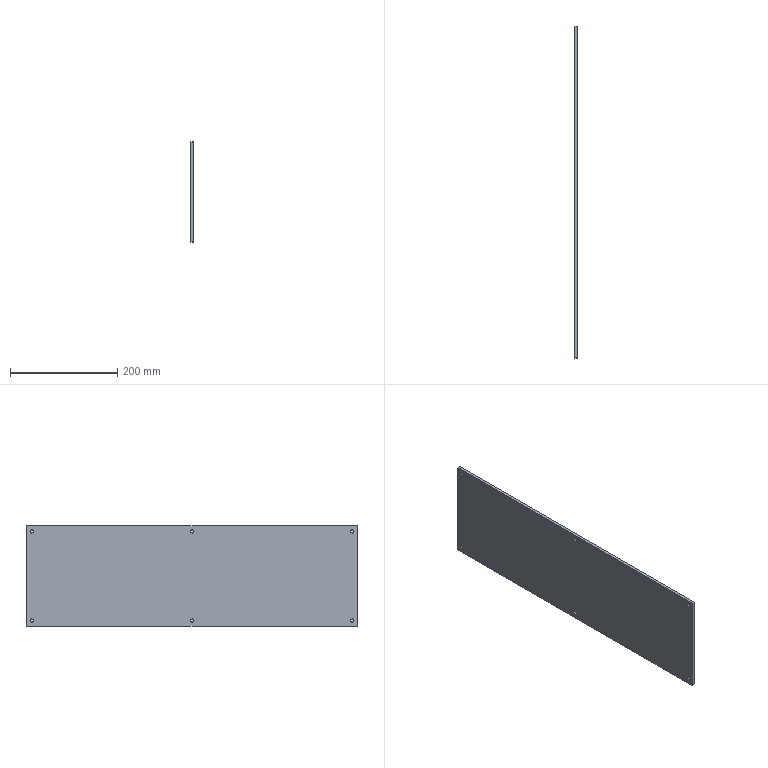Part | SolidWorks | features Chamfer 1, Extrusion 1, ICE 1 | 1 solid | 22 faces | box 5 x 618 x 188 mm | volume 580062 mm3 | cylinder 12 | plane 10 | commonest cylinder face diameters 6 x12
STEP:
#1=CARTESIAN_POINT('',(5.,0.,-86.));
#2=VERTEX_POINT('',#1);
#3=CARTESIAN_POINT('',(5.,0.,-80.));
#4=VERTEX_POINT('',#3);
#5=CARTESIAN_POINT('',(5.,0.,-83.));
#6=DIRECTION('',(-1.,0.,0.));
#7=DIRECTION('',(0.,0.,1.));
#8=AXIS2_PLACEMENT_3D('',#5,#6,#7);
#9=CIRCLE('',#8,3.);
#10=EDGE_CURVE('',#2,#4,#9,.T.);
#11=ORIENTED_EDGE('',*,*,#10,.F.);
#12=CARTESIAN_POINT('',(0.,0.,-86.));
#13=VERTEX_POINT('',#12);
#14=CARTESIAN_POINT('',(5.,0.,-86.));
#15=DIRECTION('',(-1.,0.,0.));
#16=VECTOR('',#15,1000.);
#17=LINE('',#14,#16);
#18=EDGE_CURVE('',#2,#13,#17,.T.);
#19=ORIENTED_EDGE('',*,*,#18,.T.);
#20=CARTESIAN_POINT('',(0.,0.,-80.));
#21=VERTEX_POINT('',#20);
#22=CARTESIAN_POINT('',(0.,0.,-83.));
#23=DIRECTION('',(-1.,0.,0.));
#24=DIRECTION('',(0.,0.,1.));
#25=AXIS2_PLACEMENT_3D('',#22,#23,#24);
#26=CIRCLE('',#25,3.);
#27=EDGE_CURVE('',#13,#21,#26,.T.);
#28=ORIENTED_EDGE('',*,*,#27,.T.);
#29=CARTESIAN_POINT('',(5.,0.,-80.));
#30=DIRECTION('',(-1.,0.,0.));
#31=VECTOR('',#30,1000.);
#32=LINE('',#29,#31);
#33=EDGE_CURVE('',#4,#21,#32,.T.);
#34=ORIENTED_EDGE('',*,*,#33,.F.);
#35=EDGE_LOOP('',(#11,#19,#28,#34));
#36=FACE_OUTER_BOUND('',#35,.T.);
#37=CARTESIAN_POINT('',(5.,0.,-83.));
#38=DIRECTION('',(-1.,0.,0.));
#39=DIRECTION('',(0.,0.,1.));
#40=AXIS2_PLACEMENT_3D('',#37,#38,#39);
#41=CYLINDRICAL_SURFACE('',#40,3.);
#42=ADVANCED_FACE('',(#36),#41,.F.);
#43=CARTESIAN_POINT('',(5.,0.,80.));
#44=VERTEX_POINT('',#43);
#45=CARTESIAN_POINT('',(5.,0.,86.));
#46=VERTEX_POINT('',#45);
#47=CARTESIAN_POINT('',(5.,0.,83.));
#48=DIRECTION('',(-1.,0.,0.));
#49=DIRECTION('',(0.,0.,1.));
#50=AXIS2_PLACEMENT_3D('',#47,#48,#49);
#51=CIRCLE('',#50,3.);
#52=EDGE_CURVE('',#44,#46,#51,.T.);
#53=ORIENTED_EDGE('',*,*,#52,.F.);
#54=CARTESIAN_POINT('',(0.,0.,80.));
#55=VERTEX_POINT('',#54);
#56=CARTESIAN_POINT('',(5.,0.,80.));
#57=DIRECTION('',(-1.,0.,0.));
#58=VECTOR('',#57,1000.);
#59=LINE('',#56,#58);
#60=EDGE_CURVE('',#44,#55,#59,.T.);
#61=ORIENTED_EDGE('',*,*,#60,.T.);
#62=CARTESIAN_POINT('',(0.,0.,86.));
#63=VERTEX_POINT('',#62);
#64=CARTESIAN_POINT('',(0.,0.,83.));
#65=DIRECTION('',(-1.,0.,0.));
#66=DIRECTION('',(0.,0.,1.));
#67=AXIS2_PLACEMENT_3D('',#64,#65,#66);
#68=CIRCLE('',#67,3.);
#69=EDGE_CURVE('',#55,#63,#68,.T.);
#70=ORIENTED_EDGE('',*,*,#69,.T.);
#71=CARTESIAN_POINT('',(5.,0.,86.));
#72=DIRECTION('',(-1.,0.,0.));
#73=VECTOR('',#72,1000.);
#74=LINE('',#71,#73);
#75=EDGE_CURVE('',#46,#63,#74,.T.);
#76=ORIENTED_EDGE('',*,*,#75,.F.);
#77=EDGE_LOOP('',(#53,#61,#70,#76));
#78=FACE_OUTER_BOUND('',#77,.T.);
#79=CARTESIAN_POINT('',(5.,0.,83.));
#80=DIRECTION('',(-1.,0.,0.));
#81=DIRECTION('',(0.,0.,1.));
#82=AXIS2_PLACEMENT_3D('',#79,#80,#81);
#83=CYLINDRICAL_SURFACE('',#82,3.);
#84=ADVANCED_FACE('',(#78),#83,.F.);
#85=CARTESIAN_POINT('',(5.,298.,80.));
#86=VERTEX_POINT('',#85);
#87=CARTESIAN_POINT('',(5.,298.,86.));
#88=VERTEX_POINT('',#87);
#89=CARTESIAN_POINT('',(5.,298.,83.));
#90=DIRECTION('',(-1.,0.,0.));
#91=DIRECTION('',(0.,0.,-1.));
#92=AXIS2_PLACEMENT_3D('',#89,#90,#91);
#93=CIRCLE('',#92,3.);
#94=EDGE_CURVE('',#86,#88,#93,.T.);
#95=ORIENTED_EDGE('',*,*,#94,.F.);
#96=CARTESIAN_POINT('',(0.,298.,80.));
#97=VERTEX_POINT('',#96);
#98=CARTESIAN_POINT('',(5.,298.,80.));
#99=DIRECTION('',(-1.,0.,0.));
#100=VECTOR('',#99,1000.);
#101=LINE('',#98,#100);
#102=EDGE_CURVE('',#86,#97,#101,.T.);
#103=ORIENTED_EDGE('',*,*,#102,.T.);
#104=CARTESIAN_POINT('',(0.,298.,86.));
#105=VERTEX_POINT('',#104);
#106=CARTESIAN_POINT('',(0.,298.,83.));
#107=DIRECTION('',(-1.,0.,0.));
#108=DIRECTION('',(0.,0.,-1.));
#109=AXIS2_PLACEMENT_3D('',#106,#107,#108);
#110=CIRCLE('',#109,3.);
#111=EDGE_CURVE('',#97,#105,#110,.T.);
#112=ORIENTED_EDGE('',*,*,#111,.T.);
#113=CARTESIAN_POINT('',(5.,298.,86.));
#114=DIRECTION('',(-1.,0.,0.));
#115=VECTOR('',#114,1000.);
#116=LINE('',#113,#115);
#117=EDGE_CURVE('',#88,#105,#116,.T.);
#118=ORIENTED_EDGE('',*,*,#117,.F.);
#119=EDGE_LOOP('',(#95,#103,#112,#118));
#120=FACE_OUTER_BOUND('',#119,.T.);
#121=CARTESIAN_POINT('',(5.,298.,83.));
#122=DIRECTION('',(-1.,0.,0.));
#123=DIRECTION('',(0.,0.,1.));
#124=AXIS2_PLACEMENT_3D('',#121,#122,#123);
#125=CYLINDRICAL_SURFACE('',#124,3.);
#126=ADVANCED_FACE('',(#120),#125,.F.);
#127=CARTESIAN_POINT('',(5.,-298.,80.));
#128=VERTEX_POINT('',#127);
#129=CARTESIAN_POINT('',(5.,-298.,86.));
#130=VERTEX_POINT('',#129);
#131=CARTESIAN_POINT('',(5.,-298.,83.));
#132=DIRECTION('',(-1.,0.,0.));
#133=DIRECTION('',(0.,0.,1.));
#134=AXIS2_PLACEMENT_3D('',#131,#132,#133);
#135=CIRCLE('',#134,3.);
#136=EDGE_CURVE('',#128,#130,#135,.T.);
#137=ORIENTED_EDGE('',*,*,#136,.F.);
#138=CARTESIAN_POINT('',(0.,-298.,80.));
#139=VERTEX_POINT('',#138);
#140=CARTESIAN_POINT('',(5.,-298.,80.));
#141=DIRECTION('',(-1.,0.,0.));
#142=VECTOR('',#141,1000.);
#143=LINE('',#140,#142);
#144=EDGE_CURVE('',#128,#139,#143,.T.);
#145=ORIENTED_EDGE('',*,*,#144,.T.);
#146=CARTESIAN_POINT('',(0.,-298.,86.));
#147=VERTEX_POINT('',#146);
#148=CARTESIAN_POINT('',(0.,-298.,83.));
#149=DIRECTION('',(-1.,0.,0.));
#150=DIRECTION('',(0.,0.,1.));
#151=AXIS2_PLACEMENT_3D('',#148,#149,#150);
#152=CIRCLE('',#151,3.);
#153=EDGE_CURVE('',#139,#147,#152,.T.);
#154=ORIENTED_EDGE('',*,*,#153,.T.);
#155=CARTESIAN_POINT('',(5.,-298.,86.));
#156=DIRECTION('',(-1.,0.,0.));
#157=VECTOR('',#156,1000.);
#158=LINE('',#155,#157);
#159=EDGE_CURVE('',#130,#147,#158,.T.);
#160=ORIENTED_EDGE('',*,*,#159,.F.);
#161=EDGE_LOOP('',(#137,#145,#154,#160));
#162=FACE_OUTER_BOUND('',#161,.T.);
#163=CARTESIAN_POINT('',(5.,-298.,83.));
#164=DIRECTION('',(-1.,0.,0.));
#165=DIRECTION('',(0.,0.,1.));
#166=AXIS2_PLACEMENT_3D('',#163,#164,#165);
#167=CYLINDRICAL_SURFACE('',#166,3.);
#168=ADVANCED_FACE('',(#162),#167,.F.);
#169=CARTESIAN_POINT('',(5.,-298.,-86.));
#170=VERTEX_POINT('',#169);
#171=CARTESIAN_POINT('',(5.,-298.,-80.));
#172=VERTEX_POINT('',#171);
#173=CARTESIAN_POINT('',(5.,-298.,-83.));
#174=DIRECTION('',(-1.,0.,0.));
#175=DIRECTION('',(0.,0.,-1.));
#176=AXIS2_PLACEMENT_3D('',#173,#174,#175);
#177=CIRCLE('',#176,3.);
#178=EDGE_CURVE('',#170,#172,#177,.T.);
#179=ORIENTED_EDGE('',*,*,#178,.F.);
#180=CARTESIAN_POINT('',(0.,-298.,-86.));
#181=VERTEX_POINT('',#180);
#182=CARTESIAN_POINT('',(5.,-298.,-86.));
#183=DIRECTION('',(-1.,0.,0.));
#184=VECTOR('',#183,1000.);
#185=LINE('',#182,#184);
#186=EDGE_CURVE('',#170,#181,#185,.T.);
#187=ORIENTED_EDGE('',*,*,#186,.T.);
#188=CARTESIAN_POINT('',(0.,-298.,-80.));
#189=VERTEX_POINT('',#188);
#190=CARTESIAN_POINT('',(0.,-298.,-83.));
#191=DIRECTION('',(-1.,0.,0.));
#192=DIRECTION('',(0.,0.,-1.));
#193=AXIS2_PLACEMENT_3D('',#190,#191,#192);
#194=CIRCLE('',#193,3.);
#195=EDGE_CURVE('',#181,#189,#194,.T.);
#196=ORIENTED_EDGE('',*,*,#195,.T.);
#197=CARTESIAN_POINT('',(5.,-298.,-80.));
#198=DIRECTION('',(-1.,0.,0.));
#199=VECTOR('',#198,1000.);
#200=LINE('',#197,#199);
#201=EDGE_CURVE('',#172,#189,#200,.T.);
#202=ORIENTED_EDGE('',*,*,#201,.F.);
#203=EDGE_LOOP('',(#179,#187,#196,#202));
#204=FACE_OUTER_BOUND('',#203,.T.);
#205=CARTESIAN_POINT('',(5.,-298.,-83.));
#206=DIRECTION('',(-1.,0.,0.));
#207=DIRECTION('',(0.,0.,1.));
#208=AXIS2_PLACEMENT_3D('',#205,#206,#207);
#209=CYLINDRICAL_SURFACE('',#208,3.);
#210=ADVANCED_FACE('',(#204),#209,.F.);
#211=CARTESIAN_POINT('',(5.,298.,-86.));
#212=VERTEX_POINT('',#211);
#213=CARTESIAN_POINT('',(5.,298.,-80.));
#214=VERTEX_POINT('',#213);
#215=CARTESIAN_POINT('',(5.,298.,-83.));
#216=DIRECTION('',(-1.,0.,0.));
#217=DIRECTION('',(0.,0.,1.));
#218=AXIS2_PLACEMENT_3D('',#215,#216,#217);
#219=CIRCLE('',#218,3.);
#220=EDGE_CURVE('',#212,#214,#219,.T.);
#221=ORIENTED_EDGE('',*,*,#220,.F.);
#222=CARTESIAN_POINT('',(0.,298.,-86.));
#223=VERTEX_POINT('',#222);
#224=CARTESIAN_POINT('',(5.,298.,-86.));
#225=DIRECTION('',(-1.,0.,0.));
#226=VECTOR('',#225,1000.);
#227=LINE('',#224,#226);
#228=EDGE_CURVE('',#212,#223,#227,.T.);
#229=ORIENTED_EDGE('',*,*,#228,.T.);
#230=CARTESIAN_POINT('',(0.,298.,-80.));
#231=VERTEX_POINT('',#230);
#232=CARTESIAN_POINT('',(0.,298.,-83.));
#233=DIRECTION('',(-1.,0.,0.));
#234=DIRECTION('',(0.,0.,1.));
#235=AXIS2_PLACEMENT_3D('',#232,#233,#234);
#236=CIRCLE('',#235,3.);
#237=EDGE_CURVE('',#223,#231,#236,.T.);
#238=ORIENTED_EDGE('',*,*,#237,.T.);
#239=CARTESIAN_POINT('',(5.,298.,-80.));
#240=DIRECTION('',(-1.,0.,0.));
#241=VECTOR('',#240,1000.);
#242=LINE('',#239,#241);
#243=EDGE_CURVE('',#214,#231,#242,.T.);
#244=ORIENTED_EDGE('',*,*,#243,.F.);
#245=EDGE_LOOP('',(#221,#229,#238,#244));
#246=FACE_OUTER_BOUND('',#245,.T.);
#247=CARTESIAN_POINT('',(5.,298.,-83.));
#248=DIRECTION('',(-1.,0.,0.));
#249=DIRECTION('',(0.,0.,1.));
#250=AXIS2_PLACEMENT_3D('',#247,#248,#249);
#251=CYLINDRICAL_SURFACE('',#250,3.);
#252=ADVANCED_FACE('',(#246),#251,.F.);
#253=CARTESIAN_POINT('',(0.,308.,94.));
#254=VERTEX_POINT('',#253);
#255=CARTESIAN_POINT('',(0.,-308.,94.));
#256=VERTEX_POINT('',#255);
#257=CARTESIAN_POINT('',(0.,309.,94.));
#258=DIRECTION('',(0.,-1.,0.));
#259=VECTOR('',#258,1000.);
#260=LINE('',#257,#259);
#261=EDGE_CURVE('',#254,#256,#260,.T.);
#262=ORIENTED_EDGE('',*,*,#261,.T.);
#263=CARTESIAN_POINT('',(5.,-308.,94.));
#264=VERTEX_POINT('',#263);
#265=CARTESIAN_POINT('',(5.,-308.,94.));
#266=DIRECTION('',(1.,0.,0.));
#267=VECTOR('',#266,1000.);
#268=LINE('',#265,#267);
#269=EDGE_CURVE('',#256,#264,#268,.T.);
#270=ORIENTED_EDGE('',*,*,#269,.T.);
#271=CARTESIAN_POINT('',(5.,308.,94.));
#272=VERTEX_POINT('',#271);
#273=CARTESIAN_POINT('',(5.,309.,94.));
#274=DIRECTION('',(0.,-1.,0.));
#275=VECTOR('',#274,1000.);
#276=LINE('',#273,#275);
#277=EDGE_CURVE('',#272,#264,#276,.T.);
#278=ORIENTED_EDGE('',*,*,#277,.F.);
#279=CARTESIAN_POINT('',(5.,308.,94.));
#280=DIRECTION('',(-1.,0.,0.));
#281=VECTOR('',#280,1000.);
#282=LINE('',#279,#281);
#283=EDGE_CURVE('',#272,#254,#282,.T.);
#284=ORIENTED_EDGE('',*,*,#283,.T.);
#285=EDGE_LOOP('',(#262,#270,#278,#284));
#286=FACE_OUTER_BOUND('',#285,.T.);
#287=CARTESIAN_POINT('',(5.,309.,94.));
#288=DIRECTION('',(0.,0.,-1.));
#289=DIRECTION('',(0.,1.,0.));
#290=AXIS2_PLACEMENT_3D('',#287,#288,#289);
#291=PLANE('',#290);
#292=ADVANCED_FACE('',(#286),#291,.F.);
#293=CARTESIAN_POINT('',(0.,-309.,93.));
#294=VERTEX_POINT('',#293);
#295=CARTESIAN_POINT('',(0.,-309.,-93.));
#296=VERTEX_POINT('',#295);
#297=CARTESIAN_POINT('',(0.,-309.,-94.));
#298=DIRECTION('',(0.,0.,-1.));
#299=VECTOR('',#298,1000.);
#300=LINE('',#297,#299);
#301=EDGE_CURVE('',#294,#296,#300,.T.);
#302=ORIENTED_EDGE('',*,*,#301,.T.);
#303=CARTESIAN_POINT('',(5.,-309.,-93.));
#304=VERTEX_POINT('',#303);
#305=CARTESIAN_POINT('',(5.,-309.,-93.));
#306=DIRECTION('',(1.,0.,0.));
#307=VECTOR('',#306,1000.);
#308=LINE('',#305,#307);
#309=EDGE_CURVE('',#296,#304,#308,.T.);
#310=ORIENTED_EDGE('',*,*,#309,.T.);
#311=CARTESIAN_POINT('',(5.,-309.,93.));
#312=VERTEX_POINT('',#311);
#313=CARTESIAN_POINT('',(5.,-309.,-94.));
#314=DIRECTION('',(0.,0.,-1.));
#315=VECTOR('',#314,1000.);
#316=LINE('',#313,#315);
#317=EDGE_CURVE('',#312,#304,#316,.T.);
#318=ORIENTED_EDGE('',*,*,#317,.F.);
#319=CARTESIAN_POINT('',(5.,-309.,93.));
#320=DIRECTION('',(-1.,0.,0.));
#321=VECTOR('',#320,1000.);
#322=LINE('',#319,#321);
#323=EDGE_CURVE('',#312,#294,#322,.T.);
#324=ORIENTED_EDGE('',*,*,#323,.T.);
#325=EDGE_LOOP('',(#302,#310,#318,#324));
#326=FACE_OUTER_BOUND('',#325,.T.);
#327=CARTESIAN_POINT('',(5.,-309.,-94.));
#328=DIRECTION('',(0.,1.,0.));
#329=DIRECTION('',(0.,0.,1.));
#330=AXIS2_PLACEMENT_3D('',#327,#328,#329);
#331=PLANE('',#330);
#332=ADVANCED_FACE('',(#326),#331,.F.);
#333=CARTESIAN_POINT('',(5.,-308.,-94.));
#334=VERTEX_POINT('',#333);
#335=CARTESIAN_POINT('',(5.,308.,-94.));
#336=VERTEX_POINT('',#335);
#337=CARTESIAN_POINT('',(5.,309.,-94.));
#338=DIRECTION('',(0.,1.,0.));
#339=VECTOR('',#338,1000.);
#340=LINE('',#337,#339);
#341=EDGE_CURVE('',#334,#336,#340,.T.);
#342=ORIENTED_EDGE('',*,*,#341,.F.);
#343=CARTESIAN_POINT('',(0.,-308.,-94.));
#344=VERTEX_POINT('',#343);
#345=CARTESIAN_POINT('',(5.,-308.,-94.));
#346=DIRECTION('',(-1.,0.,0.));
#347=VECTOR('',#346,1000.);
#348=LINE('',#345,#347);
#349=EDGE_CURVE('',#334,#344,#348,.T.);
#350=ORIENTED_EDGE('',*,*,#349,.T.);
#351=CARTESIAN_POINT('',(0.,308.,-94.));
#352=VERTEX_POINT('',#351);
#353=CARTESIAN_POINT('',(0.,309.,-94.));
#354=DIRECTION('',(0.,1.,0.));
#355=VECTOR('',#354,1000.);
#356=LINE('',#353,#355);
#357=EDGE_CURVE('',#344,#352,#356,.T.);
#358=ORIENTED_EDGE('',*,*,#357,.T.);
#359=CARTESIAN_POINT('',(5.,308.,-94.));
#360=DIRECTION('',(1.,0.,0.));
#361=VECTOR('',#360,1000.);
#362=LINE('',#359,#361);
#363=EDGE_CURVE('',#352,#336,#362,.T.);
#364=ORIENTED_EDGE('',*,*,#363,.T.);
#365=EDGE_LOOP('',(#342,#350,#358,#364));
#366=FACE_OUTER_BOUND('',#365,.T.);
#367=CARTESIAN_POINT('',(5.,309.,-94.));
#368=DIRECTION('',(0.,0.,1.));
#369=DIRECTION('',(0.,-1.,0.));
#370=AXIS2_PLACEMENT_3D('',#367,#368,#369);
#371=PLANE('',#370);
#372=ADVANCED_FACE('',(#366),#371,.F.);
#373=CARTESIAN_POINT('',(5.,309.,-93.));
#374=VERTEX_POINT('',#373);
#375=CARTESIAN_POINT('',(5.,309.,93.));
#376=VERTEX_POINT('',#375);
#377=CARTESIAN_POINT('',(5.,309.,-94.));
#378=DIRECTION('',(0.,0.,1.));
#379=VECTOR('',#378,1000.);
#380=LINE('',#377,#379);
#381=EDGE_CURVE('',#374,#376,#380,.T.);
#382=ORIENTED_EDGE('',*,*,#381,.F.);
#383=CARTESIAN_POINT('',(0.,309.,-93.));
#384=VERTEX_POINT('',#383);
#385=CARTESIAN_POINT('',(5.,309.,-93.));
#386=DIRECTION('',(-1.,0.,0.));
#387=VECTOR('',#386,1000.);
#388=LINE('',#385,#387);
#389=EDGE_CURVE('',#374,#384,#388,.T.);
#390=ORIENTED_EDGE('',*,*,#389,.T.);
#391=CARTESIAN_POINT('',(0.,309.,93.));
#392=VERTEX_POINT('',#391);
#393=CARTESIAN_POINT('',(0.,309.,-94.));
#394=DIRECTION('',(0.,0.,1.));
#395=VECTOR('',#394,1000.);
#396=LINE('',#393,#395);
#397=EDGE_CURVE('',#384,#392,#396,.T.);
#398=ORIENTED_EDGE('',*,*,#397,.T.);
#399=CARTESIAN_POINT('',(5.,309.,93.));
#400=DIRECTION('',(1.,0.,0.));
#401=VECTOR('',#400,1000.);
#402=LINE('',#399,#401);
#403=EDGE_CURVE('',#392,#376,#402,.T.);
#404=ORIENTED_EDGE('',*,*,#403,.T.);
#405=EDGE_LOOP('',(#382,#390,#398,#404));
#406=FACE_OUTER_BOUND('',#405,.T.);
#407=CARTESIAN_POINT('',(5.,309.,-94.));
#408=DIRECTION('',(0.,-1.,0.));
#409=DIRECTION('',(0.,0.,-1.));
#410=AXIS2_PLACEMENT_3D('',#407,#408,#409);
#411=PLANE('',#410);
#412=ADVANCED_FACE('',(#406),#411,.F.);
#413=CARTESIAN_POINT('',(5.,0.,-83.));
#414=DIRECTION('',(-1.,0.,0.));
#415=DIRECTION('',(0.,0.,1.));
#416=AXIS2_PLACEMENT_3D('',#413,#414,#415);
#417=CIRCLE('',#416,3.);
#418=EDGE_CURVE('',#4,#2,#417,.T.);
#419=ORIENTED_EDGE('',*,*,#418,.T.);
#420=ORIENTED_EDGE('',*,*,#10,.T.);
#421=EDGE_LOOP('',(#419,#420));
#422=FACE_BOUND('',#421,.T.);
#423=CARTESIAN_POINT('',(5.,0.,83.));
#424=DIRECTION('',(-1.,0.,0.));
#425=DIRECTION('',(0.,0.,1.));
#426=AXIS2_PLACEMENT_3D('',#423,#424,#425);
#427=CIRCLE('',#426,3.);
#428=EDGE_CURVE('',#46,#44,#427,.T.);
#429=ORIENTED_EDGE('',*,*,#428,.T.);
#430=ORIENTED_EDGE('',*,*,#52,.T.);
#431=EDGE_LOOP('',(#429,#430));
#432=FACE_BOUND('',#431,.T.);
#433=CARTESIAN_POINT('',(5.,298.,83.));
#434=DIRECTION('',(-1.,0.,0.));
#435=DIRECTION('',(0.,0.,-1.));
#436=AXIS2_PLACEMENT_3D('',#433,#434,#435);
#437=CIRCLE('',#436,3.);
#438=EDGE_CURVE('',#88,#86,#437,.T.);
#439=ORIENTED_EDGE('',*,*,#438,.T.);
#440=ORIENTED_EDGE('',*,*,#94,.T.);
#441=EDGE_LOOP('',(#439,#440));
#442=FACE_BOUND('',#441,.T.);
#443=CARTESIAN_POINT('',(5.,-298.,83.));
#444=DIRECTION('',(-1.,0.,0.));
#445=DIRECTION('',(0.,0.,1.));
#446=AXIS2_PLACEMENT_3D('',#443,#444,#445);
#447=CIRCLE('',#446,3.);
#448=EDGE_CURVE('',#130,#128,#447,.T.);
#449=ORIENTED_EDGE('',*,*,#448,.T.);
#450=ORIENTED_EDGE('',*,*,#136,.T.);
#451=EDGE_LOOP('',(#449,#450));
#452=FACE_BOUND('',#451,.T.);
#453=CARTESIAN_POINT('',(5.,-298.,-83.));
#454=DIRECTION('',(-1.,0.,0.));
#455=DIRECTION('',(0.,0.,-1.));
#456=AXIS2_PLACEMENT_3D('',#453,#454,#455);
#457=CIRCLE('',#456,3.);
#458=EDGE_CURVE('',#172,#170,#457,.T.);
#459=ORIENTED_EDGE('',*,*,#458,.T.);
#460=ORIENTED_EDGE('',*,*,#178,.T.);
#461=EDGE_LOOP('',(#459,#460));
#462=FACE_BOUND('',#461,.T.);
#463=CARTESIAN_POINT('',(5.,298.,-83.));
#464=DIRECTION('',(-1.,0.,0.));
#465=DIRECTION('',(0.,0.,1.));
#466=AXIS2_PLACEMENT_3D('',#463,#464,#465);
#467=CIRCLE('',#466,3.);
#468=EDGE_CURVE('',#214,#212,#467,.T.);
#469=ORIENTED_EDGE('',*,*,#468,.T.);
#470=ORIENTED_EDGE('',*,*,#220,.T.);
#471=EDGE_LOOP('',(#469,#470));
#472=FACE_BOUND('',#471,.T.);
#473=ORIENTED_EDGE('',*,*,#317,.T.);
#474=CARTESIAN_POINT('',(5.,-308.,-94.));
#475=DIRECTION('',(0.,0.7071,-0.7071));
#476=VECTOR('',#475,1000.);
#477=LINE('',#474,#476);
#478=EDGE_CURVE('',#304,#334,#477,.T.);
#479=ORIENTED_EDGE('',*,*,#478,.T.);
#480=ORIENTED_EDGE('',*,*,#341,.T.);
#481=CARTESIAN_POINT('',(5.,309.,-93.));
#482=DIRECTION('',(0.,0.7071,0.7071));
#483=VECTOR('',#482,1000.);
#484=LINE('',#481,#483);
#485=EDGE_CURVE('',#336,#374,#484,.T.);
#486=ORIENTED_EDGE('',*,*,#485,.T.);
#487=ORIENTED_EDGE('',*,*,#381,.T.);
#488=CARTESIAN_POINT('',(5.,308.,94.));
#489=DIRECTION('',(0.,-0.7071,0.7071));
#490=VECTOR('',#489,1000.);
#491=LINE('',#488,#490);
#492=EDGE_CURVE('',#376,#272,#491,.T.);
#493=ORIENTED_EDGE('',*,*,#492,.T.);
#494=ORIENTED_EDGE('',*,*,#277,.T.);
#495=CARTESIAN_POINT('',(5.,-309.,93.));
#496=DIRECTION('',(0.,-0.7071,-0.7071));
#497=VECTOR('',#496,1000.);
#498=LINE('',#495,#497);
#499=EDGE_CURVE('',#264,#312,#498,.T.);
#500=ORIENTED_EDGE('',*,*,#499,.T.);
#501=EDGE_LOOP('',(#473,#479,#480,#486,#487,#493,#494,#500));
#502=FACE_OUTER_BOUND('',#501,.T.);
#503=CARTESIAN_POINT('',(5.,-309.,94.));
#504=DIRECTION('',(-1.,0.,0.));
#505=DIRECTION('',(0.,0.,1.));
#506=AXIS2_PLACEMENT_3D('',#503,#504,#505);
#507=PLANE('',#506);
#508=ADVANCED_FACE('',(#422,#432,#442,#452,#462,#472,#502),#507,.F.);
#509=CARTESIAN_POINT('',(0.,0.,-83.));
#510=DIRECTION('',(-1.,0.,0.));
#511=DIRECTION('',(0.,0.,1.));
#512=AXIS2_PLACEMENT_3D('',#509,#510,#511);
#513=CIRCLE('',#512,3.);
#514=EDGE_CURVE('',#21,#13,#513,.T.);
#515=ORIENTED_EDGE('',*,*,#514,.F.);
#516=ORIENTED_EDGE('',*,*,#27,.F.);
#517=EDGE_LOOP('',(#515,#516));
#518=FACE_BOUND('',#517,.T.);
#519=CARTESIAN_POINT('',(0.,0.,83.));
#520=DIRECTION('',(-1.,0.,0.));
#521=DIRECTION('',(0.,0.,1.));
#522=AXIS2_PLACEMENT_3D('',#519,#520,#521);
#523=CIRCLE('',#522,3.);
#524=EDGE_CURVE('',#63,#55,#523,.T.);
#525=ORIENTED_EDGE('',*,*,#524,.F.);
#526=ORIENTED_EDGE('',*,*,#69,.F.);
#527=EDGE_LOOP('',(#525,#526));
#528=FACE_BOUND('',#527,.T.);
#529=CARTESIAN_POINT('',(0.,298.,83.));
#530=DIRECTION('',(-1.,0.,0.));
#531=DIRECTION('',(0.,0.,-1.));
#532=AXIS2_PLACEMENT_3D('',#529,#530,#531);
#533=CIRCLE('',#532,3.);
#534=EDGE_CURVE('',#105,#97,#533,.T.);
#535=ORIENTED_EDGE('',*,*,#534,.F.);
#536=ORIENTED_EDGE('',*,*,#111,.F.);
#537=EDGE_LOOP('',(#535,#536));
#538=FACE_BOUND('',#537,.T.);
#539=CARTESIAN_POINT('',(0.,-298.,83.));
#540=DIRECTION('',(-1.,0.,0.));
#541=DIRECTION('',(0.,0.,1.));
#542=AXIS2_PLACEMENT_3D('',#539,#540,#541);
#543=CIRCLE('',#542,3.);
#544=EDGE_CURVE('',#147,#139,#543,.T.);
#545=ORIENTED_EDGE('',*,*,#544,.F.);
#546=ORIENTED_EDGE('',*,*,#153,.F.);
#547=EDGE_LOOP('',(#545,#546));
#548=FACE_BOUND('',#547,.T.);
#549=CARTESIAN_POINT('',(0.,-298.,-83.));
#550=DIRECTION('',(-1.,0.,0.));
#551=DIRECTION('',(0.,0.,-1.));
#552=AXIS2_PLACEMENT_3D('',#549,#550,#551);
#553=CIRCLE('',#552,3.);
#554=EDGE_CURVE('',#189,#181,#553,.T.);
#555=ORIENTED_EDGE('',*,*,#554,.F.);
#556=ORIENTED_EDGE('',*,*,#195,.F.);
#557=EDGE_LOOP('',(#555,#556));
#558=FACE_BOUND('',#557,.T.);
#559=CARTESIAN_POINT('',(0.,298.,-83.));
#560=DIRECTION('',(-1.,0.,0.));
#561=DIRECTION('',(0.,0.,1.));
#562=AXIS2_PLACEMENT_3D('',#559,#560,#561);
#563=CIRCLE('',#562,3.);
#564=EDGE_CURVE('',#231,#223,#563,.T.);
#565=ORIENTED_EDGE('',*,*,#564,.F.);
#566=ORIENTED_EDGE('',*,*,#237,.F.);
#567=EDGE_LOOP('',(#565,#566));
#568=FACE_BOUND('',#567,.T.);
#569=ORIENTED_EDGE('',*,*,#357,.F.);
#570=CARTESIAN_POINT('',(0.,-402.5,0.5));
#571=DIRECTION('',(0.,-0.7071,0.7071));
#572=VECTOR('',#571,1000.);
#573=LINE('',#570,#572);
#574=EDGE_CURVE('',#344,#296,#573,.T.);
#575=ORIENTED_EDGE('',*,*,#574,.T.);
#576=ORIENTED_EDGE('',*,*,#301,.F.);
#577=CARTESIAN_POINT('',(0.,-308.5,93.5));
#578=DIRECTION('',(0.,0.7071,0.7071));
#579=VECTOR('',#578,1000.);
#580=LINE('',#577,#579);
#581=EDGE_CURVE('',#294,#256,#580,.T.);
#582=ORIENTED_EDGE('',*,*,#581,.T.);
#583=ORIENTED_EDGE('',*,*,#261,.F.);
#584=CARTESIAN_POINT('',(0.,-0.5,402.5));
#585=DIRECTION('',(0.,0.7071,-0.7071));
#586=VECTOR('',#585,1000.);
#587=LINE('',#584,#586);
#588=EDGE_CURVE('',#254,#392,#587,.T.);
#589=ORIENTED_EDGE('',*,*,#588,.T.);
#590=ORIENTED_EDGE('',*,*,#397,.F.);
#591=CARTESIAN_POINT('',(0.,93.5,-308.5));
#592=DIRECTION('',(0.,-0.7071,-0.7071));
#593=VECTOR('',#592,1000.);
#594=LINE('',#591,#593);
#595=EDGE_CURVE('',#384,#352,#594,.T.);
#596=ORIENTED_EDGE('',*,*,#595,.T.);
#597=EDGE_LOOP('',(#569,#575,#576,#582,#583,#589,#590,#596));
#598=FACE_OUTER_BOUND('',#597,.T.);
#599=CARTESIAN_POINT('',(0.,-309.,94.));
#600=DIRECTION('',(-1.,0.,0.));
#601=DIRECTION('',(0.,0.,1.));
#602=AXIS2_PLACEMENT_3D('',#599,#600,#601);
#603=PLANE('',#602);
#604=ADVANCED_FACE('',(#518,#528,#538,#548,#558,#568,#598),#603,.T.);
#605=ORIENTED_EDGE('',*,*,#478,.F.);
#606=ORIENTED_EDGE('',*,*,#309,.F.);
#607=ORIENTED_EDGE('',*,*,#574,.F.);
#608=ORIENTED_EDGE('',*,*,#349,.F.);
#609=EDGE_LOOP('',(#605,#606,#607,#608));
#610=FACE_OUTER_BOUND('',#609,.T.);
#611=CARTESIAN_POINT('',(5.,-308.,-94.));
#612=DIRECTION('',(0.,0.7071,0.7071));
#613=DIRECTION('',(0.,-0.7071,0.7071));
#614=AXIS2_PLACEMENT_3D('',#611,#612,#613);
#615=PLANE('',#614);
#616=ADVANCED_FACE('',(#610),#615,.F.);
#617=ORIENTED_EDGE('',*,*,#499,.F.);
#618=ORIENTED_EDGE('',*,*,#269,.F.);
#619=ORIENTED_EDGE('',*,*,#581,.F.);
#620=ORIENTED_EDGE('',*,*,#323,.F.);
#621=EDGE_LOOP('',(#617,#618,#619,#620));
#622=FACE_OUTER_BOUND('',#621,.T.);
#623=CARTESIAN_POINT('',(5.,-309.,93.));
#624=DIRECTION('',(0.,0.7071,-0.7071));
#625=DIRECTION('',(0.,0.7071,0.7071));
#626=AXIS2_PLACEMENT_3D('',#623,#624,#625);
#627=PLANE('',#626);
#628=ADVANCED_FACE('',(#622),#627,.F.);
#629=ORIENTED_EDGE('',*,*,#485,.F.);
#630=ORIENTED_EDGE('',*,*,#363,.F.);
#631=ORIENTED_EDGE('',*,*,#595,.F.);
#632=ORIENTED_EDGE('',*,*,#389,.F.);
#633=EDGE_LOOP('',(#629,#630,#631,#632));
#634=FACE_OUTER_BOUND('',#633,.T.);
#635=CARTESIAN_POINT('',(5.,309.,-93.));
#636=DIRECTION('',(0.,-0.7071,0.7071));
#637=DIRECTION('',(0.,-0.7071,-0.7071));
#638=AXIS2_PLACEMENT_3D('',#635,#636,#637);
#639=PLANE('',#638);
#640=ADVANCED_FACE('',(#634),#639,.F.);
#641=ORIENTED_EDGE('',*,*,#492,.F.);
#642=ORIENTED_EDGE('',*,*,#403,.F.);
#643=ORIENTED_EDGE('',*,*,#588,.F.);
#644=ORIENTED_EDGE('',*,*,#283,.F.);
#645=EDGE_LOOP('',(#641,#642,#643,#644));
#646=FACE_OUTER_BOUND('',#645,.T.);
#647=CARTESIAN_POINT('',(5.,308.,94.));
#648=DIRECTION('',(0.,-0.7071,-0.7071));
#649=DIRECTION('',(0.,0.7071,-0.7071));
#650=AXIS2_PLACEMENT_3D('',#647,#648,#649);
#651=PLANE('',#650);
#652=ADVANCED_FACE('',(#646),#651,.F.);
#653=ORIENTED_EDGE('',*,*,#228,.F.);
#654=ORIENTED_EDGE('',*,*,#468,.F.);
#655=ORIENTED_EDGE('',*,*,#243,.T.);
#656=ORIENTED_EDGE('',*,*,#564,.T.);
#657=EDGE_LOOP('',(#653,#654,#655,#656));
#658=FACE_OUTER_BOUND('',#657,.T.);
#659=CARTESIAN_POINT('',(5.,298.,-83.));
#660=DIRECTION('',(-1.,0.,0.));
#661=DIRECTION('',(0.,0.,1.));
#662=AXIS2_PLACEMENT_3D('',#659,#660,#661);
#663=CYLINDRICAL_SURFACE('',#662,3.);
#664=ADVANCED_FACE('',(#658),#663,.F.);
#665=ORIENTED_EDGE('',*,*,#186,.F.);
#666=ORIENTED_EDGE('',*,*,#458,.F.);
#667=ORIENTED_EDGE('',*,*,#201,.T.);
#668=ORIENTED_EDGE('',*,*,#554,.T.);
#669=EDGE_LOOP('',(#665,#666,#667,#668));
#670=FACE_OUTER_BOUND('',#669,.T.);
#671=CARTESIAN_POINT('',(5.,-298.,-83.));
#672=DIRECTION('',(-1.,0.,0.));
#673=DIRECTION('',(0.,0.,1.));
#674=AXIS2_PLACEMENT_3D('',#671,#672,#673);
#675=CYLINDRICAL_SURFACE('',#674,3.);
#676=ADVANCED_FACE('',(#670),#675,.F.);
#677=ORIENTED_EDGE('',*,*,#144,.F.);
#678=ORIENTED_EDGE('',*,*,#448,.F.);
#679=ORIENTED_EDGE('',*,*,#159,.T.);
#680=ORIENTED_EDGE('',*,*,#544,.T.);
#681=EDGE_LOOP('',(#677,#678,#679,#680));
#682=FACE_OUTER_BOUND('',#681,.T.);
#683=CARTESIAN_POINT('',(5.,-298.,83.));
#684=DIRECTION('',(-1.,0.,0.));
#685=DIRECTION('',(0.,0.,1.));
#686=AXIS2_PLACEMENT_3D('',#683,#684,#685);
#687=CYLINDRICAL_SURFACE('',#686,3.);
#688=ADVANCED_FACE('',(#682),#687,.F.);
#689=ORIENTED_EDGE('',*,*,#102,.F.);
#690=ORIENTED_EDGE('',*,*,#438,.F.);
#691=ORIENTED_EDGE('',*,*,#117,.T.);
#692=ORIENTED_EDGE('',*,*,#534,.T.);
#693=EDGE_LOOP('',(#689,#690,#691,#692));
#694=FACE_OUTER_BOUND('',#693,.T.);
#695=CARTESIAN_POINT('',(5.,298.,83.));
#696=DIRECTION('',(-1.,0.,0.));
#697=DIRECTION('',(0.,0.,1.));
#698=AXIS2_PLACEMENT_3D('',#695,#696,#697);
#699=CYLINDRICAL_SURFACE('',#698,3.);
#700=ADVANCED_FACE('',(#694),#699,.F.);
#701=ORIENTED_EDGE('',*,*,#60,.F.);
#702=ORIENTED_EDGE('',*,*,#428,.F.);
#703=ORIENTED_EDGE('',*,*,#75,.T.);
#704=ORIENTED_EDGE('',*,*,#524,.T.);
#705=EDGE_LOOP('',(#701,#702,#703,#704));
#706=FACE_OUTER_BOUND('',#705,.T.);
#707=CARTESIAN_POINT('',(5.,0.,83.));
#708=DIRECTION('',(-1.,0.,0.));
#709=DIRECTION('',(0.,0.,1.));
#710=AXIS2_PLACEMENT_3D('',#707,#708,#709);
#711=CYLINDRICAL_SURFACE('',#710,3.);
#712=ADVANCED_FACE('',(#706),#711,.F.);
#713=ORIENTED_EDGE('',*,*,#18,.F.);
#714=ORIENTED_EDGE('',*,*,#418,.F.);
#715=ORIENTED_EDGE('',*,*,#33,.T.);
#716=ORIENTED_EDGE('',*,*,#514,.T.);
#717=EDGE_LOOP('',(#713,#714,#715,#716));
#718=FACE_OUTER_BOUND('',#717,.T.);
#719=CARTESIAN_POINT('',(5.,0.,-83.));
#720=DIRECTION('',(-1.,0.,0.));
#721=DIRECTION('',(0.,0.,1.));
#722=AXIS2_PLACEMENT_3D('',#719,#720,#721);
#723=CYLINDRICAL_SURFACE('',#722,3.);
#724=ADVANCED_FACE('',(#718),#723,.F.);
#725=CLOSED_SHELL('',(#42,#84,#126,#168,#210,#252,#292,#332,#372,#412,#508,#604,#616,#628,#640,#652,#664,#676,#688,#700,#712,#724));
#726=MANIFOLD_SOLID_BREP('',#725);
#727=CARTESIAN_POINT('',(0.,0.,0.));
#728=DIRECTION('',(0.,0.,1.));
#729=DIRECTION('',(1.,0.,0.));
#730=AXIS2_PLACEMENT_3D('',#727,#728,#729);
#731=(LENGTH_UNIT()NAMED_UNIT(*)SI_UNIT(.MILLI.,.METRE.));
#732=UNCERTAINTY_MEASURE_WITH_UNIT(LENGTH_MEASURE(0.00001),#731,'','');
#733=(NAMED_UNIT(*)PLANE_ANGLE_UNIT()SI_UNIT($,.RADIAN.));
#734=(NAMED_UNIT(*)SI_UNIT($,.STERADIAN.)SOLID_ANGLE_UNIT());
#735=(GEOMETRIC_REPRESENTATION_CONTEXT(3)GLOBAL_UNCERTAINTY_ASSIGNED_CONTEXT((#732))GLOBAL_UNIT_ASSIGNED_CONTEXT((#731,#733,#734))REPRESENTATION_CONTEXT('',''));
#736=ADVANCED_BREP_SHAPE_REPRESENTATION('',(#726,#730),#735);